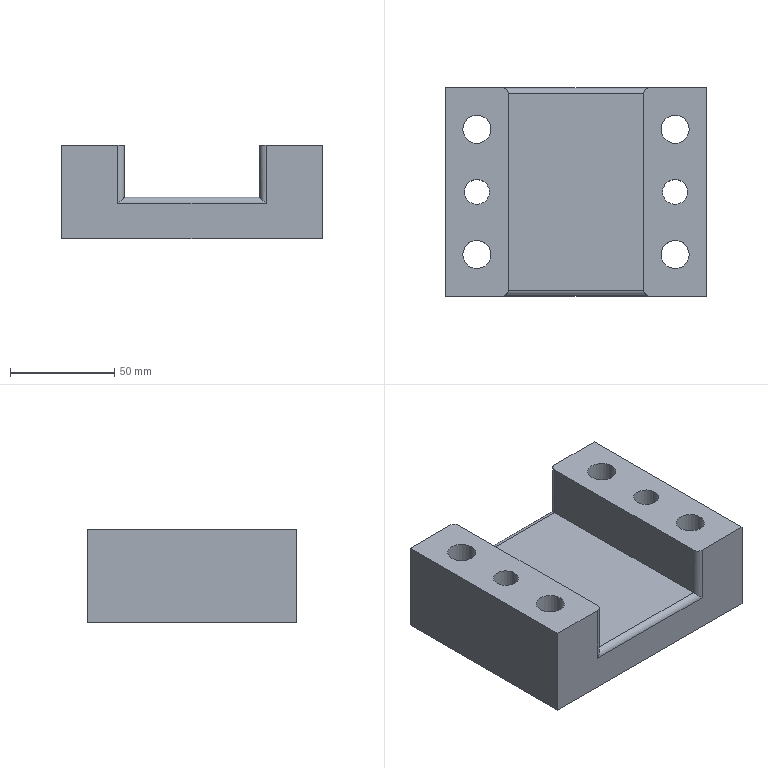Part | NX | features MAIN_BODY 2 | 1 solid | 30 faces | box 125 x 100 x 45 mm | volume 346500 mm3 | cylinder 16 | plane 14 | commonest cylinder face diameters 6 x6 13.5 x4 20 x4 12 x2
STEP:
#1=CARTESIAN_POINT('',(-437.,15.,377.));
#2=VERTEX_POINT('',#1);
#3=CARTESIAN_POINT('',(-508.,15.,377.));
#4=VERTEX_POINT('',#3);
#5=CARTESIAN_POINT('',(-440.,15.,377.));
#6=DIRECTION('',(-1.,0.,0.));
#7=VECTOR('',#6,1000.);
#8=LINE('',#5,#7);
#9=EDGE_CURVE('',#2,#4,#8,.T.);
#10=ORIENTED_EDGE('',*,*,#9,.F.);
#11=CARTESIAN_POINT('',(-437.,15.,405.));
#12=VERTEX_POINT('',#11);
#13=CARTESIAN_POINT('',(-437.,15.,380.));
#14=DIRECTION('',(0.,0.,1.));
#15=VECTOR('',#14,1000.);
#16=LINE('',#13,#15);
#17=EDGE_CURVE('',#12,#2,#16,.F.);
#18=ORIENTED_EDGE('',*,*,#17,.F.);
#19=CARTESIAN_POINT('',(-410.,15.,405.));
#20=VERTEX_POINT('',#19);
#21=CARTESIAN_POINT('',(-505.,15.,405.));
#22=DIRECTION('',(1.,0.,0.));
#23=VECTOR('',#22,1000.);
#24=LINE('',#21,#23);
#25=EDGE_CURVE('',#12,#20,#24,.T.);
#26=ORIENTED_EDGE('',*,*,#25,.T.);
#27=CARTESIAN_POINT('',(-410.,15.,360.));
#28=VERTEX_POINT('',#27);
#29=CARTESIAN_POINT('',(-410.,15.,380.));
#30=DIRECTION('',(0.,0.,1.));
#31=VECTOR('',#30,1000.);
#32=LINE('',#29,#31);
#33=EDGE_CURVE('',#20,#28,#32,.F.);
#34=ORIENTED_EDGE('',*,*,#33,.T.);
#35=CARTESIAN_POINT('',(-535.,15.,360.));
#36=VERTEX_POINT('',#35);
#37=CARTESIAN_POINT('',(-440.,15.,360.));
#38=DIRECTION('',(-1.,0.,0.));
#39=VECTOR('',#38,1000.);
#40=LINE('',#37,#39);
#41=EDGE_CURVE('',#28,#36,#40,.T.);
#42=ORIENTED_EDGE('',*,*,#41,.T.);
#43=CARTESIAN_POINT('',(-535.,15.,405.));
#44=VERTEX_POINT('',#43);
#45=CARTESIAN_POINT('',(-535.,15.,380.));
#46=DIRECTION('',(0.,0.,-1.));
#47=VECTOR('',#46,1000.);
#48=LINE('',#45,#47);
#49=EDGE_CURVE('',#44,#36,#48,.T.);
#50=ORIENTED_EDGE('',*,*,#49,.F.);
#51=CARTESIAN_POINT('',(-508.,15.,405.));
#52=VERTEX_POINT('',#51);
#53=CARTESIAN_POINT('',(-505.,15.,405.));
#54=DIRECTION('',(1.,0.,0.));
#55=VECTOR('',#54,1000.);
#56=LINE('',#53,#55);
#57=EDGE_CURVE('',#52,#44,#56,.F.);
#58=ORIENTED_EDGE('',*,*,#57,.F.);
#59=CARTESIAN_POINT('',(-508.,15.,405.));
#60=DIRECTION('',(0.,0.,1.));
#61=VECTOR('',#60,1000.);
#62=LINE('',#59,#61);
#63=EDGE_CURVE('',#4,#52,#62,.T.);
#64=ORIENTED_EDGE('',*,*,#63,.F.);
#65=EDGE_LOOP('',(#10,#18,#26,#34,#42,#50,#58,#64));
#66=FACE_BOUND('',#65,.T.);
#67=CARTESIAN_POINT('',(-440.,15.,380.));
#68=DIRECTION('',(0.,1.,0.));
#69=DIRECTION('',(-1.,0.,0.));
#70=AXIS2_PLACEMENT_3D('',#67,#68,#69);
#71=PLANE('',#70);
#72=ADVANCED_FACE('',(#66),#71,.T.);
#73=CARTESIAN_POINT('',(-508.,-85.,377.));
#74=VERTEX_POINT('',#73);
#75=CARTESIAN_POINT('',(-437.,-85.,377.));
#76=VERTEX_POINT('',#75);
#77=CARTESIAN_POINT('',(-440.,-85.,377.));
#78=DIRECTION('',(-1.,0.,0.));
#79=VECTOR('',#78,1000.);
#80=LINE('',#77,#79);
#81=EDGE_CURVE('',#74,#76,#80,.F.);
#82=ORIENTED_EDGE('',*,*,#81,.F.);
#83=CARTESIAN_POINT('',(-508.,-85.,405.));
#84=VERTEX_POINT('',#83);
#85=CARTESIAN_POINT('',(-508.,-85.,380.));
#86=DIRECTION('',(0.,0.,1.));
#87=VECTOR('',#86,1000.);
#88=LINE('',#85,#87);
#89=EDGE_CURVE('',#84,#74,#88,.F.);
#90=ORIENTED_EDGE('',*,*,#89,.F.);
#91=CARTESIAN_POINT('',(-535.,-85.,405.));
#92=VERTEX_POINT('',#91);
#93=CARTESIAN_POINT('',(-440.,-85.,405.));
#94=DIRECTION('',(-1.,0.,0.));
#95=VECTOR('',#94,1000.);
#96=LINE('',#93,#95);
#97=EDGE_CURVE('',#84,#92,#96,.T.);
#98=ORIENTED_EDGE('',*,*,#97,.T.);
#99=CARTESIAN_POINT('',(-535.,-85.,360.));
#100=VERTEX_POINT('',#99);
#101=CARTESIAN_POINT('',(-535.,-85.,380.));
#102=DIRECTION('',(0.,0.,-1.));
#103=VECTOR('',#102,1000.);
#104=LINE('',#101,#103);
#105=EDGE_CURVE('',#92,#100,#104,.T.);
#106=ORIENTED_EDGE('',*,*,#105,.T.);
#107=CARTESIAN_POINT('',(-410.,-85.,360.));
#108=VERTEX_POINT('',#107);
#109=CARTESIAN_POINT('',(-440.,-85.,360.));
#110=DIRECTION('',(1.,0.,0.));
#111=VECTOR('',#110,1000.);
#112=LINE('',#109,#111);
#113=EDGE_CURVE('',#108,#100,#112,.F.);
#114=ORIENTED_EDGE('',*,*,#113,.F.);
#115=CARTESIAN_POINT('',(-410.,-85.,405.));
#116=VERTEX_POINT('',#115);
#117=CARTESIAN_POINT('',(-410.,-85.,380.));
#118=DIRECTION('',(0.,0.,-1.));
#119=VECTOR('',#118,1000.);
#120=LINE('',#117,#119);
#121=EDGE_CURVE('',#116,#108,#120,.T.);
#122=ORIENTED_EDGE('',*,*,#121,.F.);
#123=CARTESIAN_POINT('',(-437.,-85.,405.));
#124=VERTEX_POINT('',#123);
#125=CARTESIAN_POINT('',(-440.,-85.,405.));
#126=DIRECTION('',(-1.,0.,0.));
#127=VECTOR('',#126,1000.);
#128=LINE('',#125,#127);
#129=EDGE_CURVE('',#124,#116,#128,.F.);
#130=ORIENTED_EDGE('',*,*,#129,.F.);
#131=CARTESIAN_POINT('',(-437.,-85.,405.));
#132=DIRECTION('',(0.,0.,1.));
#133=VECTOR('',#132,1000.);
#134=LINE('',#131,#133);
#135=EDGE_CURVE('',#76,#124,#134,.T.);
#136=ORIENTED_EDGE('',*,*,#135,.F.);
#137=EDGE_LOOP('',(#82,#90,#98,#106,#114,#122,#130,#136));
#138=FACE_BOUND('',#137,.T.);
#139=CARTESIAN_POINT('',(-440.,-85.,380.));
#140=DIRECTION('',(0.,1.,0.));
#141=DIRECTION('',(-1.,0.,0.));
#142=AXIS2_PLACEMENT_3D('',#139,#140,#141);
#143=PLANE('',#142);
#144=ADVANCED_FACE('',(#138),#143,.F.);
#145=CARTESIAN_POINT('',(-526.,-35.,360.));
#146=VERTEX_POINT('',#145);
#147=CARTESIAN_POINT('',(-520.,-35.,360.));
#148=DIRECTION('',(0.,0.,-1.));
#149=DIRECTION('',(-1.,0.,0.));
#150=AXIS2_PLACEMENT_3D('',#147,#148,#149);
#151=CIRCLE('',#150,6.);
#152=EDGE_CURVE('',#146,#146,#151,.T.);
#153=ORIENTED_EDGE('',*,*,#152,.F.);
#154=EDGE_LOOP('',(#153));
#155=FACE_BOUND('',#154,.T.);
#156=CARTESIAN_POINT('',(-431.,-35.,360.));
#157=VERTEX_POINT('',#156);
#158=CARTESIAN_POINT('',(-425.,-35.,360.));
#159=DIRECTION('',(0.,0.,-1.));
#160=DIRECTION('',(-1.,0.,0.));
#161=AXIS2_PLACEMENT_3D('',#158,#159,#160);
#162=CIRCLE('',#161,6.);
#163=EDGE_CURVE('',#157,#157,#162,.T.);
#164=ORIENTED_EDGE('',*,*,#163,.F.);
#165=EDGE_LOOP('',(#164));
#166=FACE_BOUND('',#165,.T.);
#167=CARTESIAN_POINT('',(-415.,-65.,360.));
#168=VERTEX_POINT('',#167);
#169=CARTESIAN_POINT('',(-425.,-65.,360.));
#170=DIRECTION('',(0.,0.,1.));
#171=DIRECTION('',(1.,0.,0.));
#172=AXIS2_PLACEMENT_3D('',#169,#170,#171);
#173=CIRCLE('',#172,10.);
#174=EDGE_CURVE('',#168,#168,#173,.T.);
#175=ORIENTED_EDGE('',*,*,#174,.T.);
#176=EDGE_LOOP('',(#175));
#177=FACE_BOUND('',#176,.T.);
#178=CARTESIAN_POINT('',(-415.,-5.,360.));
#179=VERTEX_POINT('',#178);
#180=CARTESIAN_POINT('',(-425.,-5.,360.));
#181=DIRECTION('',(0.,0.,1.));
#182=DIRECTION('',(1.,0.,0.));
#183=AXIS2_PLACEMENT_3D('',#180,#181,#182);
#184=CIRCLE('',#183,10.);
#185=EDGE_CURVE('',#179,#179,#184,.T.);
#186=ORIENTED_EDGE('',*,*,#185,.T.);
#187=EDGE_LOOP('',(#186));
#188=FACE_BOUND('',#187,.T.);
#189=CARTESIAN_POINT('',(-510.,-5.,360.));
#190=VERTEX_POINT('',#189);
#191=CARTESIAN_POINT('',(-520.,-5.,360.));
#192=DIRECTION('',(0.,0.,1.));
#193=DIRECTION('',(1.,0.,0.));
#194=AXIS2_PLACEMENT_3D('',#191,#192,#193);
#195=CIRCLE('',#194,10.);
#196=EDGE_CURVE('',#190,#190,#195,.T.);
#197=ORIENTED_EDGE('',*,*,#196,.T.);
#198=EDGE_LOOP('',(#197));
#199=FACE_BOUND('',#198,.T.);
#200=CARTESIAN_POINT('',(-510.,-65.,360.));
#201=VERTEX_POINT('',#200);
#202=CARTESIAN_POINT('',(-520.,-65.,360.));
#203=DIRECTION('',(0.,0.,1.));
#204=DIRECTION('',(1.,0.,0.));
#205=AXIS2_PLACEMENT_3D('',#202,#203,#204);
#206=CIRCLE('',#205,10.);
#207=EDGE_CURVE('',#201,#201,#206,.T.);
#208=ORIENTED_EDGE('',*,*,#207,.T.);
#209=EDGE_LOOP('',(#208));
#210=FACE_BOUND('',#209,.T.);
#211=ORIENTED_EDGE('',*,*,#113,.T.);
#212=CARTESIAN_POINT('',(-535.,-5.,360.));
#213=DIRECTION('',(0.,1.,0.));
#214=VECTOR('',#213,1000.);
#215=LINE('',#212,#214);
#216=EDGE_CURVE('',#36,#100,#215,.F.);
#217=ORIENTED_EDGE('',*,*,#216,.F.);
#218=ORIENTED_EDGE('',*,*,#41,.F.);
#219=CARTESIAN_POINT('',(-410.,-5.,360.));
#220=DIRECTION('',(0.,1.,0.));
#221=VECTOR('',#220,1000.);
#222=LINE('',#219,#221);
#223=EDGE_CURVE('',#28,#108,#222,.F.);
#224=ORIENTED_EDGE('',*,*,#223,.T.);
#225=EDGE_LOOP('',(#211,#217,#218,#224));
#226=FACE_BOUND('',#225,.T.);
#227=CARTESIAN_POINT('',(-440.,-5.,360.));
#228=DIRECTION('',(0.,0.,1.));
#229=DIRECTION('',(1.,0.,0.));
#230=AXIS2_PLACEMENT_3D('',#227,#228,#229);
#231=PLANE('',#230);
#232=ADVANCED_FACE('',(#155,#166,#177,#188,#199,#210,#226),#231,.F.);
#233=CARTESIAN_POINT('',(-440.,12.,380.));
#234=VERTEX_POINT('',#233);
#235=CARTESIAN_POINT('',(-440.,-82.,380.));
#236=VERTEX_POINT('',#235);
#237=CARTESIAN_POINT('',(-440.,-5.,380.));
#238=DIRECTION('',(0.,1.,0.));
#239=VECTOR('',#238,1000.);
#240=LINE('',#237,#239);
#241=EDGE_CURVE('',#234,#236,#240,.F.);
#242=ORIENTED_EDGE('',*,*,#241,.F.);
#243=CARTESIAN_POINT('',(-505.,12.,380.));
#244=VERTEX_POINT('',#243);
#245=CARTESIAN_POINT('',(-440.,12.,380.));
#246=DIRECTION('',(-1.,0.,0.));
#247=VECTOR('',#246,1000.);
#248=LINE('',#245,#247);
#249=EDGE_CURVE('',#244,#234,#248,.F.);
#250=ORIENTED_EDGE('',*,*,#249,.F.);
#251=CARTESIAN_POINT('',(-505.,-82.,380.));
#252=VERTEX_POINT('',#251);
#253=CARTESIAN_POINT('',(-505.,-361.5,380.));
#254=DIRECTION('',(0.,1.,0.));
#255=VECTOR('',#254,1000.);
#256=LINE('',#253,#255);
#257=EDGE_CURVE('',#244,#252,#256,.F.);
#258=ORIENTED_EDGE('',*,*,#257,.T.);
#259=CARTESIAN_POINT('',(-440.,-82.,380.));
#260=DIRECTION('',(1.,0.,0.));
#261=VECTOR('',#260,1000.);
#262=LINE('',#259,#261);
#263=EDGE_CURVE('',#236,#252,#262,.F.);
#264=ORIENTED_EDGE('',*,*,#263,.F.);
#265=EDGE_LOOP('',(#242,#250,#258,#264));
#266=FACE_BOUND('',#265,.T.);
#267=CARTESIAN_POINT('',(-440.,-5.,380.));
#268=DIRECTION('',(0.,0.,1.));
#269=DIRECTION('',(1.,0.,0.));
#270=AXIS2_PLACEMENT_3D('',#267,#268,#269);
#271=PLANE('',#270);
#272=ADVANCED_FACE('',(#266),#271,.T.);
#273=CARTESIAN_POINT('',(-440.,12.,405.));
#274=VERTEX_POINT('',#273);
#275=CARTESIAN_POINT('',(-440.,-82.,405.));
#276=VERTEX_POINT('',#275);
#277=CARTESIAN_POINT('',(-440.,363.5,405.));
#278=DIRECTION('',(0.,1.,0.));
#279=VECTOR('',#278,1000.);
#280=LINE('',#277,#279);
#281=EDGE_CURVE('',#274,#276,#280,.F.);
#282=ORIENTED_EDGE('',*,*,#281,.F.);
#283=CARTESIAN_POINT('',(-440.,12.,405.));
#284=DIRECTION('',(0.,0.,-1.));
#285=VECTOR('',#284,1000.);
#286=LINE('',#283,#285);
#287=EDGE_CURVE('',#234,#274,#286,.F.);
#288=ORIENTED_EDGE('',*,*,#287,.F.);
#289=ORIENTED_EDGE('',*,*,#241,.T.);
#290=CARTESIAN_POINT('',(-440.,-82.,380.));
#291=DIRECTION('',(0.,0.,1.));
#292=VECTOR('',#291,1000.);
#293=LINE('',#290,#292);
#294=EDGE_CURVE('',#276,#236,#293,.F.);
#295=ORIENTED_EDGE('',*,*,#294,.F.);
#296=EDGE_LOOP('',(#282,#288,#289,#295));
#297=FACE_BOUND('',#296,.T.);
#298=CARTESIAN_POINT('',(-440.,363.5,405.));
#299=DIRECTION('',(-1.,0.,0.));
#300=DIRECTION('',(0.,0.,1.));
#301=AXIS2_PLACEMENT_3D('',#298,#299,#300);
#302=PLANE('',#301);
#303=ADVANCED_FACE('',(#297),#302,.T.);
#304=CARTESIAN_POINT('',(-431.,-35.,405.));
#305=VERTEX_POINT('',#304);
#306=CARTESIAN_POINT('',(-425.,-35.,405.));
#307=DIRECTION('',(0.,0.,-1.));
#308=DIRECTION('',(-1.,0.,0.));
#309=AXIS2_PLACEMENT_3D('',#306,#307,#308);
#310=CIRCLE('',#309,6.);
#311=EDGE_CURVE('',#305,#305,#310,.T.);
#312=ORIENTED_EDGE('',*,*,#311,.T.);
#313=EDGE_LOOP('',(#312));
#314=FACE_BOUND('',#313,.T.);
#315=CARTESIAN_POINT('',(-431.75,-65.,405.));
#316=VERTEX_POINT('',#315);
#317=CARTESIAN_POINT('',(-425.,-65.,405.));
#318=DIRECTION('',(0.,0.,-1.));
#319=DIRECTION('',(-1.,0.,0.));
#320=AXIS2_PLACEMENT_3D('',#317,#318,#319);
#321=CIRCLE('',#320,6.75);
#322=EDGE_CURVE('',#316,#316,#321,.F.);
#323=ORIENTED_EDGE('',*,*,#322,.F.);
#324=EDGE_LOOP('',(#323));
#325=FACE_BOUND('',#324,.T.);
#326=CARTESIAN_POINT('',(-431.75,-5.,405.));
#327=VERTEX_POINT('',#326);
#328=CARTESIAN_POINT('',(-425.,-5.,405.));
#329=DIRECTION('',(0.,0.,-1.));
#330=DIRECTION('',(-1.,0.,0.));
#331=AXIS2_PLACEMENT_3D('',#328,#329,#330);
#332=CIRCLE('',#331,6.75);
#333=EDGE_CURVE('',#327,#327,#332,.F.);
#334=ORIENTED_EDGE('',*,*,#333,.F.);
#335=EDGE_LOOP('',(#334));
#336=FACE_BOUND('',#335,.T.);
#337=ORIENTED_EDGE('',*,*,#129,.T.);
#338=CARTESIAN_POINT('',(-410.,363.5,405.));
#339=DIRECTION('',(0.,1.,0.));
#340=VECTOR('',#339,1000.);
#341=LINE('',#338,#340);
#342=EDGE_CURVE('',#20,#116,#341,.F.);
#343=ORIENTED_EDGE('',*,*,#342,.F.);
#344=ORIENTED_EDGE('',*,*,#25,.F.);
#345=CARTESIAN_POINT('',(-437.,12.,405.));
#346=DIRECTION('',(0.,0.,-1.));
#347=DIRECTION('',(-1.,0.,0.));
#348=AXIS2_PLACEMENT_3D('',#345,#346,#347);
#349=CIRCLE('',#348,3.);
#350=EDGE_CURVE('',#274,#12,#349,.T.);
#351=ORIENTED_EDGE('',*,*,#350,.F.);
#352=ORIENTED_EDGE('',*,*,#281,.T.);
#353=CARTESIAN_POINT('',(-437.,-82.,405.));
#354=DIRECTION('',(0.,0.,-1.));
#355=DIRECTION('',(-1.,0.,0.));
#356=AXIS2_PLACEMENT_3D('',#353,#354,#355);
#357=CIRCLE('',#356,3.);
#358=EDGE_CURVE('',#124,#276,#357,.T.);
#359=ORIENTED_EDGE('',*,*,#358,.F.);
#360=EDGE_LOOP('',(#337,#343,#344,#351,#352,#359));
#361=FACE_BOUND('',#360,.T.);
#362=CARTESIAN_POINT('',(-505.,363.5,405.));
#363=DIRECTION('',(0.,0.,1.));
#364=DIRECTION('',(1.,0.,0.));
#365=AXIS2_PLACEMENT_3D('',#362,#363,#364);
#366=PLANE('',#365);
#367=ADVANCED_FACE('',(#314,#325,#336,#361),#366,.T.);
#368=ORIENTED_EDGE('',*,*,#33,.F.);
#369=ORIENTED_EDGE('',*,*,#342,.T.);
#370=ORIENTED_EDGE('',*,*,#121,.T.);
#371=ORIENTED_EDGE('',*,*,#223,.F.);
#372=EDGE_LOOP('',(#368,#369,#370,#371));
#373=FACE_BOUND('',#372,.T.);
#374=CARTESIAN_POINT('',(-410.,-5.,380.));
#375=DIRECTION('',(-1.,0.,0.));
#376=DIRECTION('',(0.,-1.,0.));
#377=AXIS2_PLACEMENT_3D('',#374,#375,#376);
#378=PLANE('',#377);
#379=ADVANCED_FACE('',(#373),#378,.F.);
#380=CARTESIAN_POINT('',(-526.,-35.,405.));
#381=VERTEX_POINT('',#380);
#382=CARTESIAN_POINT('',(-520.,-35.,405.));
#383=DIRECTION('',(0.,0.,-1.));
#384=DIRECTION('',(-1.,0.,0.));
#385=AXIS2_PLACEMENT_3D('',#382,#383,#384);
#386=CIRCLE('',#385,6.);
#387=EDGE_CURVE('',#381,#381,#386,.F.);
#388=ORIENTED_EDGE('',*,*,#387,.F.);
#389=EDGE_LOOP('',(#388));
#390=FACE_BOUND('',#389,.T.);
#391=CARTESIAN_POINT('',(-526.75,-5.,405.));
#392=VERTEX_POINT('',#391);
#393=CARTESIAN_POINT('',(-520.,-5.,405.));
#394=DIRECTION('',(0.,0.,-1.));
#395=DIRECTION('',(-1.,0.,0.));
#396=AXIS2_PLACEMENT_3D('',#393,#394,#395);
#397=CIRCLE('',#396,6.75);
#398=EDGE_CURVE('',#392,#392,#397,.T.);
#399=ORIENTED_EDGE('',*,*,#398,.T.);
#400=EDGE_LOOP('',(#399));
#401=FACE_BOUND('',#400,.T.);
#402=CARTESIAN_POINT('',(-526.75,-65.,405.));
#403=VERTEX_POINT('',#402);
#404=CARTESIAN_POINT('',(-520.,-65.,405.));
#405=DIRECTION('',(0.,0.,-1.));
#406=DIRECTION('',(-1.,0.,0.));
#407=AXIS2_PLACEMENT_3D('',#404,#405,#406);
#408=CIRCLE('',#407,6.75);
#409=EDGE_CURVE('',#403,#403,#408,.T.);
#410=ORIENTED_EDGE('',*,*,#409,.T.);
#411=EDGE_LOOP('',(#410));
#412=FACE_BOUND('',#411,.T.);
#413=CARTESIAN_POINT('',(-505.,12.,405.));
#414=VERTEX_POINT('',#413);
#415=CARTESIAN_POINT('',(-505.,-82.,405.));
#416=VERTEX_POINT('',#415);
#417=CARTESIAN_POINT('',(-505.,363.5,405.));
#418=DIRECTION('',(0.,-1.,0.));
#419=VECTOR('',#418,1000.);
#420=LINE('',#417,#419);
#421=EDGE_CURVE('',#414,#416,#420,.T.);
#422=ORIENTED_EDGE('',*,*,#421,.F.);
#423=CARTESIAN_POINT('',(-508.,12.,405.));
#424=DIRECTION('',(0.,0.,-1.));
#425=DIRECTION('',(-1.,0.,0.));
#426=AXIS2_PLACEMENT_3D('',#423,#424,#425);
#427=CIRCLE('',#426,3.);
#428=EDGE_CURVE('',#52,#414,#427,.T.);
#429=ORIENTED_EDGE('',*,*,#428,.F.);
#430=ORIENTED_EDGE('',*,*,#57,.T.);
#431=CARTESIAN_POINT('',(-535.,363.5,405.));
#432=DIRECTION('',(0.,1.,0.));
#433=VECTOR('',#432,1000.);
#434=LINE('',#431,#433);
#435=EDGE_CURVE('',#44,#92,#434,.F.);
#436=ORIENTED_EDGE('',*,*,#435,.T.);
#437=ORIENTED_EDGE('',*,*,#97,.F.);
#438=CARTESIAN_POINT('',(-508.,-82.,405.));
#439=DIRECTION('',(0.,0.,-1.));
#440=DIRECTION('',(-1.,0.,0.));
#441=AXIS2_PLACEMENT_3D('',#438,#439,#440);
#442=CIRCLE('',#441,3.);
#443=EDGE_CURVE('',#416,#84,#442,.T.);
#444=ORIENTED_EDGE('',*,*,#443,.F.);
#445=EDGE_LOOP('',(#422,#429,#430,#436,#437,#444));
#446=FACE_BOUND('',#445,.T.);
#447=CARTESIAN_POINT('',(-505.,363.5,405.));
#448=DIRECTION('',(0.,0.,1.));
#449=DIRECTION('',(1.,0.,0.));
#450=AXIS2_PLACEMENT_3D('',#447,#448,#449);
#451=PLANE('',#450);
#452=ADVANCED_FACE('',(#390,#401,#412,#446),#451,.T.);
#453=ORIENTED_EDGE('',*,*,#257,.F.);
#454=CARTESIAN_POINT('',(-505.,12.,380.));
#455=DIRECTION('',(0.,0.,-1.));
#456=VECTOR('',#455,1000.);
#457=LINE('',#454,#456);
#458=EDGE_CURVE('',#414,#244,#457,.T.);
#459=ORIENTED_EDGE('',*,*,#458,.F.);
#460=ORIENTED_EDGE('',*,*,#421,.T.);
#461=CARTESIAN_POINT('',(-505.,-82.,405.));
#462=DIRECTION('',(0.,0.,1.));
#463=VECTOR('',#462,1000.);
#464=LINE('',#461,#463);
#465=EDGE_CURVE('',#252,#416,#464,.T.);
#466=ORIENTED_EDGE('',*,*,#465,.F.);
#467=EDGE_LOOP('',(#453,#459,#460,#466));
#468=FACE_BOUND('',#467,.T.);
#469=CARTESIAN_POINT('',(-505.,-361.5,405.));
#470=DIRECTION('',(1.,0.,0.));
#471=DIRECTION('',(0.,0.,-1.));
#472=AXIS2_PLACEMENT_3D('',#469,#470,#471);
#473=PLANE('',#472);
#474=ADVANCED_FACE('',(#468),#473,.T.);
#475=ORIENTED_EDGE('',*,*,#435,.F.);
#476=ORIENTED_EDGE('',*,*,#49,.T.);
#477=ORIENTED_EDGE('',*,*,#216,.T.);
#478=ORIENTED_EDGE('',*,*,#105,.F.);
#479=EDGE_LOOP('',(#475,#476,#477,#478));
#480=FACE_BOUND('',#479,.T.);
#481=CARTESIAN_POINT('',(-535.,-5.,380.));
#482=DIRECTION('',(-1.,0.,0.));
#483=DIRECTION('',(0.,-1.,0.));
#484=AXIS2_PLACEMENT_3D('',#481,#482,#483);
#485=PLANE('',#484);
#486=ADVANCED_FACE('',(#480),#485,.T.);
#487=CARTESIAN_POINT('',(-513.25,-65.,385.));
#488=VERTEX_POINT('',#487);
#489=CARTESIAN_POINT('',(-520.,-65.,385.));
#490=DIRECTION('',(0.,0.,1.));
#491=DIRECTION('',(1.,0.,0.));
#492=AXIS2_PLACEMENT_3D('',#489,#490,#491);
#493=CIRCLE('',#492,6.75);
#494=EDGE_CURVE('',#488,#488,#493,.T.);
#495=ORIENTED_EDGE('',*,*,#494,.F.);
#496=EDGE_LOOP('',(#495));
#497=FACE_BOUND('',#496,.T.);
#498=ORIENTED_EDGE('',*,*,#409,.F.);
#499=EDGE_LOOP('',(#498));
#500=FACE_BOUND('',#499,.T.);
#501=CARTESIAN_POINT('',(-520.,-65.,460.));
#502=DIRECTION('',(0.,0.,1.));
#503=DIRECTION('',(1.,0.,0.));
#504=AXIS2_PLACEMENT_3D('',#501,#502,#503);
#505=CYLINDRICAL_SURFACE('',#504,6.75);
#506=ADVANCED_FACE('',(#497,#500),#505,.F.);
#507=ORIENTED_EDGE('',*,*,#494,.T.);
#508=EDGE_LOOP('',(#507));
#509=FACE_BOUND('',#508,.T.);
#510=CARTESIAN_POINT('',(-510.,-65.,385.));
#511=VERTEX_POINT('',#510);
#512=CARTESIAN_POINT('',(-520.,-65.,385.));
#513=DIRECTION('',(0.,0.,1.));
#514=DIRECTION('',(1.,0.,0.));
#515=AXIS2_PLACEMENT_3D('',#512,#513,#514);
#516=CIRCLE('',#515,10.);
#517=EDGE_CURVE('',#511,#511,#516,.T.);
#518=ORIENTED_EDGE('',*,*,#517,.F.);
#519=EDGE_LOOP('',(#518));
#520=FACE_BOUND('',#519,.T.);
#521=CARTESIAN_POINT('',(-519.,-65.,385.));
#522=DIRECTION('',(0.,0.,1.));
#523=DIRECTION('',(1.,0.,0.));
#524=AXIS2_PLACEMENT_3D('',#521,#522,#523);
#525=PLANE('',#524);
#526=ADVANCED_FACE('',(#509,#520),#525,.F.);
#527=ORIENTED_EDGE('',*,*,#517,.T.);
#528=EDGE_LOOP('',(#527));
#529=FACE_BOUND('',#528,.T.);
#530=ORIENTED_EDGE('',*,*,#207,.F.);
#531=EDGE_LOOP('',(#530));
#532=FACE_BOUND('',#531,.T.);
#533=CARTESIAN_POINT('',(-520.,-65.,360.));
#534=DIRECTION('',(0.,0.,1.));
#535=DIRECTION('',(1.,0.,0.));
#536=AXIS2_PLACEMENT_3D('',#533,#534,#535);
#537=CYLINDRICAL_SURFACE('',#536,10.);
#538=ADVANCED_FACE('',(#529,#532),#537,.F.);
#539=CARTESIAN_POINT('',(-513.25,-5.,385.));
#540=VERTEX_POINT('',#539);
#541=CARTESIAN_POINT('',(-520.,-5.,385.));
#542=DIRECTION('',(0.,0.,1.));
#543=DIRECTION('',(1.,0.,0.));
#544=AXIS2_PLACEMENT_3D('',#541,#542,#543);
#545=CIRCLE('',#544,6.75);
#546=EDGE_CURVE('',#540,#540,#545,.T.);
#547=ORIENTED_EDGE('',*,*,#546,.F.);
#548=EDGE_LOOP('',(#547));
#549=FACE_BOUND('',#548,.T.);
#550=ORIENTED_EDGE('',*,*,#398,.F.);
#551=EDGE_LOOP('',(#550));
#552=FACE_BOUND('',#551,.T.);
#553=CARTESIAN_POINT('',(-520.,-5.,460.));
#554=DIRECTION('',(0.,0.,1.));
#555=DIRECTION('',(1.,0.,0.));
#556=AXIS2_PLACEMENT_3D('',#553,#554,#555);
#557=CYLINDRICAL_SURFACE('',#556,6.75);
#558=ADVANCED_FACE('',(#549,#552),#557,.F.);
#559=ORIENTED_EDGE('',*,*,#546,.T.);
#560=EDGE_LOOP('',(#559));
#561=FACE_BOUND('',#560,.T.);
#562=CARTESIAN_POINT('',(-510.,-5.,385.));
#563=VERTEX_POINT('',#562);
#564=CARTESIAN_POINT('',(-520.,-5.,385.));
#565=DIRECTION('',(0.,0.,1.));
#566=DIRECTION('',(1.,0.,0.));
#567=AXIS2_PLACEMENT_3D('',#564,#565,#566);
#568=CIRCLE('',#567,10.);
#569=EDGE_CURVE('',#563,#563,#568,.T.);
#570=ORIENTED_EDGE('',*,*,#569,.F.);
#571=EDGE_LOOP('',(#570));
#572=FACE_BOUND('',#571,.T.);
#573=CARTESIAN_POINT('',(-519.,-5.,385.));
#574=DIRECTION('',(0.,0.,1.));
#575=DIRECTION('',(1.,0.,0.));
#576=AXIS2_PLACEMENT_3D('',#573,#574,#575);
#577=PLANE('',#576);
#578=ADVANCED_FACE('',(#561,#572),#577,.F.);
#579=ORIENTED_EDGE('',*,*,#569,.T.);
#580=EDGE_LOOP('',(#579));
#581=FACE_BOUND('',#580,.T.);
#582=ORIENTED_EDGE('',*,*,#196,.F.);
#583=EDGE_LOOP('',(#582));
#584=FACE_BOUND('',#583,.T.);
#585=CARTESIAN_POINT('',(-520.,-5.,360.));
#586=DIRECTION('',(0.,0.,1.));
#587=DIRECTION('',(1.,0.,0.));
#588=AXIS2_PLACEMENT_3D('',#585,#586,#587);
#589=CYLINDRICAL_SURFACE('',#588,10.);
#590=ADVANCED_FACE('',(#581,#584),#589,.F.);
#591=ORIENTED_EDGE('',*,*,#333,.T.);
#592=EDGE_LOOP('',(#591));
#593=FACE_BOUND('',#592,.T.);
#594=CARTESIAN_POINT('',(-418.25,-5.,385.));
#595=VERTEX_POINT('',#594);
#596=CARTESIAN_POINT('',(-425.,-5.,385.));
#597=DIRECTION('',(0.,0.,1.));
#598=DIRECTION('',(1.,0.,0.));
#599=AXIS2_PLACEMENT_3D('',#596,#597,#598);
#600=CIRCLE('',#599,6.75);
#601=EDGE_CURVE('',#595,#595,#600,.T.);
#602=ORIENTED_EDGE('',*,*,#601,.F.);
#603=EDGE_LOOP('',(#602));
#604=FACE_BOUND('',#603,.T.);
#605=CARTESIAN_POINT('',(-425.,-5.,460.));
#606=DIRECTION('',(0.,0.,1.));
#607=DIRECTION('',(1.,0.,0.));
#608=AXIS2_PLACEMENT_3D('',#605,#606,#607);
#609=CYLINDRICAL_SURFACE('',#608,6.75);
#610=ADVANCED_FACE('',(#593,#604),#609,.F.);
#611=ORIENTED_EDGE('',*,*,#601,.T.);
#612=EDGE_LOOP('',(#611));
#613=FACE_BOUND('',#612,.T.);
#614=CARTESIAN_POINT('',(-415.,-5.,385.));
#615=VERTEX_POINT('',#614);
#616=CARTESIAN_POINT('',(-425.,-5.,385.));
#617=DIRECTION('',(0.,0.,1.));
#618=DIRECTION('',(1.,0.,0.));
#619=AXIS2_PLACEMENT_3D('',#616,#617,#618);
#620=CIRCLE('',#619,10.);
#621=EDGE_CURVE('',#615,#615,#620,.T.);
#622=ORIENTED_EDGE('',*,*,#621,.F.);
#623=EDGE_LOOP('',(#622));
#624=FACE_BOUND('',#623,.T.);
#625=CARTESIAN_POINT('',(-426.,-5.,385.));
#626=DIRECTION('',(0.,0.,1.));
#627=DIRECTION('',(1.,0.,0.));
#628=AXIS2_PLACEMENT_3D('',#625,#626,#627);
#629=PLANE('',#628);
#630=ADVANCED_FACE('',(#613,#624),#629,.F.);
#631=ORIENTED_EDGE('',*,*,#621,.T.);
#632=EDGE_LOOP('',(#631));
#633=FACE_BOUND('',#632,.T.);
#634=ORIENTED_EDGE('',*,*,#185,.F.);
#635=EDGE_LOOP('',(#634));
#636=FACE_BOUND('',#635,.T.);
#637=CARTESIAN_POINT('',(-425.,-5.,360.));
#638=DIRECTION('',(0.,0.,1.));
#639=DIRECTION('',(1.,0.,0.));
#640=AXIS2_PLACEMENT_3D('',#637,#638,#639);
#641=CYLINDRICAL_SURFACE('',#640,10.);
#642=ADVANCED_FACE('',(#633,#636),#641,.F.);
#643=ORIENTED_EDGE('',*,*,#322,.T.);
#644=EDGE_LOOP('',(#643));
#645=FACE_BOUND('',#644,.T.);
#646=CARTESIAN_POINT('',(-418.25,-65.,385.));
#647=VERTEX_POINT('',#646);
#648=CARTESIAN_POINT('',(-425.,-65.,385.));
#649=DIRECTION('',(0.,0.,1.));
#650=DIRECTION('',(1.,0.,0.));
#651=AXIS2_PLACEMENT_3D('',#648,#649,#650);
#652=CIRCLE('',#651,6.75);
#653=EDGE_CURVE('',#647,#647,#652,.T.);
#654=ORIENTED_EDGE('',*,*,#653,.F.);
#655=EDGE_LOOP('',(#654));
#656=FACE_BOUND('',#655,.T.);
#657=CARTESIAN_POINT('',(-425.,-65.,460.));
#658=DIRECTION('',(0.,0.,1.));
#659=DIRECTION('',(1.,0.,0.));
#660=AXIS2_PLACEMENT_3D('',#657,#658,#659);
#661=CYLINDRICAL_SURFACE('',#660,6.75);
#662=ADVANCED_FACE('',(#645,#656),#661,.F.);
#663=ORIENTED_EDGE('',*,*,#653,.T.);
#664=EDGE_LOOP('',(#663));
#665=FACE_BOUND('',#664,.T.);
#666=CARTESIAN_POINT('',(-415.,-65.,385.));
#667=VERTEX_POINT('',#666);
#668=CARTESIAN_POINT('',(-425.,-65.,385.));
#669=DIRECTION('',(0.,0.,1.));
#670=DIRECTION('',(1.,0.,0.));
#671=AXIS2_PLACEMENT_3D('',#668,#669,#670);
#672=CIRCLE('',#671,10.);
#673=EDGE_CURVE('',#667,#667,#672,.T.);
#674=ORIENTED_EDGE('',*,*,#673,.F.);
#675=EDGE_LOOP('',(#674));
#676=FACE_BOUND('',#675,.T.);
#677=CARTESIAN_POINT('',(-426.,-65.,385.));
#678=DIRECTION('',(0.,0.,1.));
#679=DIRECTION('',(1.,0.,0.));
#680=AXIS2_PLACEMENT_3D('',#677,#678,#679);
#681=PLANE('',#680);
#682=ADVANCED_FACE('',(#665,#676),#681,.F.);
#683=ORIENTED_EDGE('',*,*,#673,.T.);
#684=EDGE_LOOP('',(#683));
#685=FACE_BOUND('',#684,.T.);
#686=ORIENTED_EDGE('',*,*,#174,.F.);
#687=EDGE_LOOP('',(#686));
#688=FACE_BOUND('',#687,.T.);
#689=CARTESIAN_POINT('',(-425.,-65.,360.));
#690=DIRECTION('',(0.,0.,1.));
#691=DIRECTION('',(1.,0.,0.));
#692=AXIS2_PLACEMENT_3D('',#689,#690,#691);
#693=CYLINDRICAL_SURFACE('',#692,10.);
#694=ADVANCED_FACE('',(#685,#688),#693,.F.);
#695=ORIENTED_EDGE('',*,*,#311,.F.);
#696=EDGE_LOOP('',(#695));
#697=FACE_BOUND('',#696,.T.);
#698=ORIENTED_EDGE('',*,*,#163,.T.);
#699=EDGE_LOOP('',(#698));
#700=FACE_BOUND('',#699,.T.);
#701=CARTESIAN_POINT('',(-425.,-35.,360.));
#702=DIRECTION('',(0.,0.,1.));
#703=DIRECTION('',(-1.,0.,0.));
#704=AXIS2_PLACEMENT_3D('',#701,#702,#703);
#705=CYLINDRICAL_SURFACE('',#704,6.);
#706=ADVANCED_FACE('',(#697,#700),#705,.F.);
#707=ORIENTED_EDGE('',*,*,#152,.T.);
#708=EDGE_LOOP('',(#707));
#709=FACE_BOUND('',#708,.T.);
#710=ORIENTED_EDGE('',*,*,#387,.T.);
#711=EDGE_LOOP('',(#710));
#712=FACE_BOUND('',#711,.T.);
#713=CARTESIAN_POINT('',(-520.,-35.,360.));
#714=DIRECTION('',(0.,0.,1.));
#715=DIRECTION('',(-1.,0.,0.));
#716=AXIS2_PLACEMENT_3D('',#713,#714,#715);
#717=CYLINDRICAL_SURFACE('',#716,6.);
#718=ADVANCED_FACE('',(#709,#712),#717,.F.);
#719=ORIENTED_EDGE('',*,*,#443,.T.);
#720=ORIENTED_EDGE('',*,*,#89,.T.);
#721=CARTESIAN_POINT('',(-508.,-82.,377.));
#722=DIRECTION('',(-0.7071,0.,0.7071));
#723=DIRECTION('',(0.7071,0.,0.7071));
#724=AXIS2_PLACEMENT_3D('',#721,#722,#723);
#725=ELLIPSE('',#724,4.243,3.);
#726=EDGE_CURVE('',#74,#252,#725,.T.);
#727=ORIENTED_EDGE('',*,*,#726,.T.);
#728=ORIENTED_EDGE('',*,*,#465,.T.);
#729=EDGE_LOOP('',(#719,#720,#727,#728));
#730=FACE_BOUND('',#729,.T.);
#731=CARTESIAN_POINT('',(-508.,-82.,380.));
#732=DIRECTION('',(0.,0.,1.));
#733=DIRECTION('',(-1.,0.,0.));
#734=AXIS2_PLACEMENT_3D('',#731,#732,#733);
#735=CYLINDRICAL_SURFACE('',#734,3.);
#736=ADVANCED_FACE('',(#730),#735,.T.);
#737=ORIENTED_EDGE('',*,*,#726,.F.);
#738=ORIENTED_EDGE('',*,*,#81,.T.);
#739=CARTESIAN_POINT('',(-437.,-82.,377.));
#740=DIRECTION('',(-0.7071,0.,-0.7071));
#741=DIRECTION('',(-0.7071,0.,0.7071));
#742=AXIS2_PLACEMENT_3D('',#739,#740,#741);
#743=ELLIPSE('',#742,4.243,3.);
#744=EDGE_CURVE('',#76,#236,#743,.T.);
#745=ORIENTED_EDGE('',*,*,#744,.T.);
#746=ORIENTED_EDGE('',*,*,#263,.T.);
#747=EDGE_LOOP('',(#737,#738,#745,#746));
#748=FACE_BOUND('',#747,.T.);
#749=CARTESIAN_POINT('',(-440.,-82.,377.));
#750=DIRECTION('',(1.,0.,0.));
#751=DIRECTION('',(0.,0.,1.));
#752=AXIS2_PLACEMENT_3D('',#749,#750,#751);
#753=CYLINDRICAL_SURFACE('',#752,3.);
#754=ADVANCED_FACE('',(#748),#753,.T.);
#755=ORIENTED_EDGE('',*,*,#358,.T.);
#756=ORIENTED_EDGE('',*,*,#294,.T.);
#757=ORIENTED_EDGE('',*,*,#744,.F.);
#758=ORIENTED_EDGE('',*,*,#135,.T.);
#759=EDGE_LOOP('',(#755,#756,#757,#758));
#760=FACE_BOUND('',#759,.T.);
#761=CARTESIAN_POINT('',(-437.,-82.,405.));
#762=DIRECTION('',(0.,0.,1.));
#763=DIRECTION('',(-1.,0.,0.));
#764=AXIS2_PLACEMENT_3D('',#761,#762,#763);
#765=CYLINDRICAL_SURFACE('',#764,3.);
#766=ADVANCED_FACE('',(#760),#765,.T.);
#767=ORIENTED_EDGE('',*,*,#350,.T.);
#768=ORIENTED_EDGE('',*,*,#17,.T.);
#769=CARTESIAN_POINT('',(-437.,12.,377.));
#770=DIRECTION('',(0.7071,0.,0.7071));
#771=DIRECTION('',(0.7071,0.,-0.7071));
#772=AXIS2_PLACEMENT_3D('',#769,#770,#771);
#773=ELLIPSE('',#772,4.243,3.);
#774=EDGE_CURVE('',#2,#234,#773,.T.);
#775=ORIENTED_EDGE('',*,*,#774,.T.);
#776=ORIENTED_EDGE('',*,*,#287,.T.);
#777=EDGE_LOOP('',(#767,#768,#775,#776));
#778=FACE_BOUND('',#777,.T.);
#779=CARTESIAN_POINT('',(-437.,12.,380.));
#780=DIRECTION('',(0.,0.,-1.));
#781=DIRECTION('',(1.,0.,0.));
#782=AXIS2_PLACEMENT_3D('',#779,#780,#781);
#783=CYLINDRICAL_SURFACE('',#782,3.);
#784=ADVANCED_FACE('',(#778),#783,.T.);
#785=ORIENTED_EDGE('',*,*,#774,.F.);
#786=ORIENTED_EDGE('',*,*,#9,.T.);
#787=CARTESIAN_POINT('',(-508.,12.,377.));
#788=DIRECTION('',(-0.7071,0.,0.7071));
#789=DIRECTION('',(-0.7071,0.,-0.7071));
#790=AXIS2_PLACEMENT_3D('',#787,#788,#789);
#791=ELLIPSE('',#790,4.243,3.);
#792=EDGE_CURVE('',#4,#244,#791,.F.);
#793=ORIENTED_EDGE('',*,*,#792,.T.);
#794=ORIENTED_EDGE('',*,*,#249,.T.);
#795=EDGE_LOOP('',(#785,#786,#793,#794));
#796=FACE_BOUND('',#795,.T.);
#797=CARTESIAN_POINT('',(-440.,12.,377.));
#798=DIRECTION('',(-1.,0.,0.));
#799=DIRECTION('',(0.,0.,-1.));
#800=AXIS2_PLACEMENT_3D('',#797,#798,#799);
#801=CYLINDRICAL_SURFACE('',#800,3.);
#802=ADVANCED_FACE('',(#796),#801,.T.);
#803=ORIENTED_EDGE('',*,*,#428,.T.);
#804=ORIENTED_EDGE('',*,*,#458,.T.);
#805=ORIENTED_EDGE('',*,*,#792,.F.);
#806=ORIENTED_EDGE('',*,*,#63,.T.);
#807=EDGE_LOOP('',(#803,#804,#805,#806));
#808=FACE_BOUND('',#807,.T.);
#809=CARTESIAN_POINT('',(-508.,12.,405.));
#810=DIRECTION('',(0.,0.,-1.));
#811=DIRECTION('',(1.,0.,0.));
#812=AXIS2_PLACEMENT_3D('',#809,#810,#811);
#813=CYLINDRICAL_SURFACE('',#812,3.);
#814=ADVANCED_FACE('',(#808),#813,.T.);
#815=CLOSED_SHELL('',(#72,#144,#232,#272,#303,#367,#379,#452,#474,#486,#506,#526,#538,#558,#578,#590,#610,#630,#642,#662,#682,#694,#706,#718,#736,#754,#766,#784,#802,#814));
#816=MANIFOLD_SOLID_BREP('',#815);
#817=(LENGTH_UNIT()NAMED_UNIT(*)SI_UNIT(.MILLI.,.METRE.));
#818=UNCERTAINTY_MEASURE_WITH_UNIT(LENGTH_MEASURE(0.00001),#817,'','');
#819=(NAMED_UNIT(*)PLANE_ANGLE_UNIT()SI_UNIT($,.RADIAN.));
#820=(NAMED_UNIT(*)SI_UNIT($,.STERADIAN.)SOLID_ANGLE_UNIT());
#821=(GEOMETRIC_REPRESENTATION_CONTEXT(3)GLOBAL_UNCERTAINTY_ASSIGNED_CONTEXT((#818))GLOBAL_UNIT_ASSIGNED_CONTEXT((#817,#819,#820))REPRESENTATION_CONTEXT('',''));
#822=ADVANCED_BREP_SHAPE_REPRESENTATION('',(#816),#821);